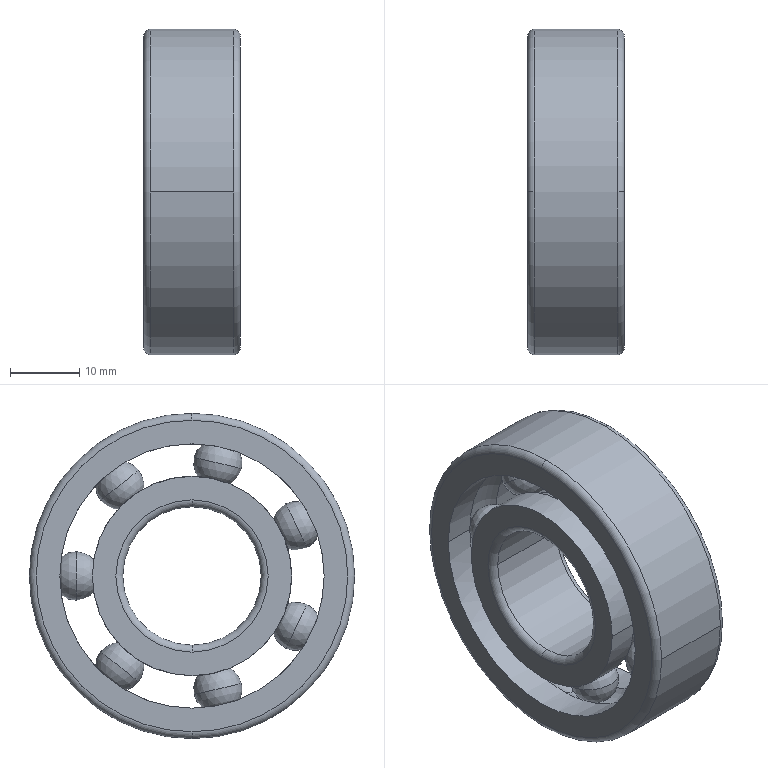Part | STEP file | KS B 2023 - 6204 - 20 x 47 x 14 | 9 solids | 65 faces | box 14 x 47 x 47 mm | volume 13264 mm3 | torus 35 | sphere 14 | cylinder 12 | plane 4 | commonest cylinder face diameters 28.802 x4 38.198 x4 20 x2 47 x2